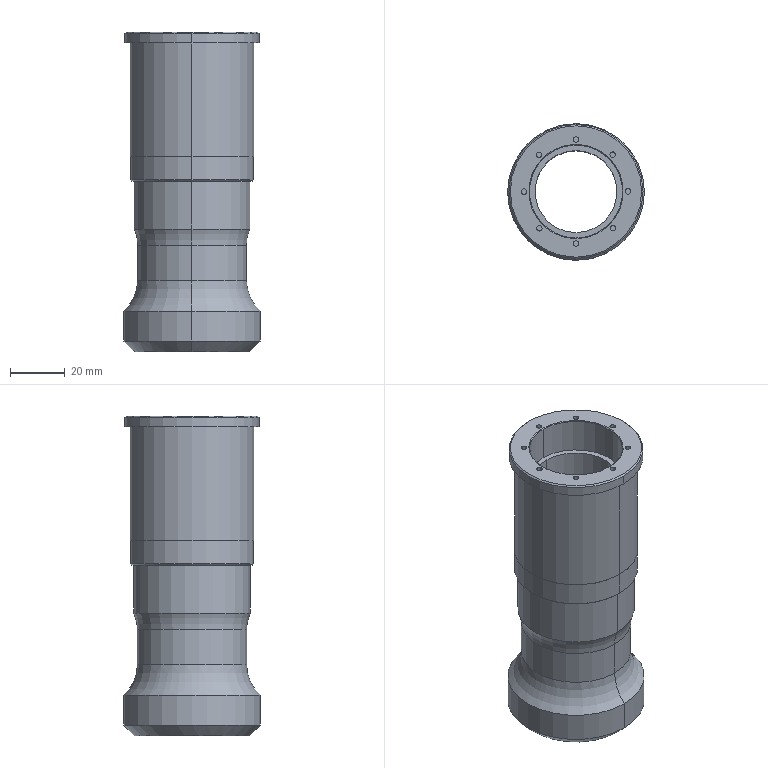Part | STEP file | 2026.6.15-Main Assembly图.sldasm-Part-98 | 1 solid | 86 faces | box 50 x 50 x 116.9 mm | volume 92626 mm3 | cylinder 50 | plane 22 | cone 10 | torus 4 | commonest cylinder face diameters 2 x32 34 x4 30 x2 40 x2 42.5 x2 44.9 x2